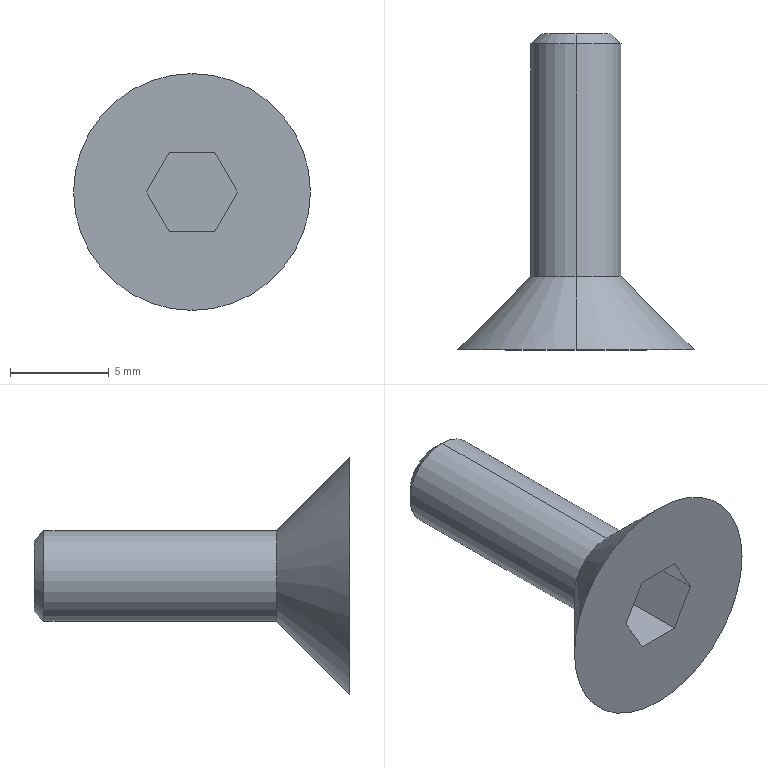Part | CATIA | 1 solid | 15 faces | box 12 x 16 x 12 mm | volume 370.466 mm3 | plane 9 | cone 4 | cylinder 2 | commonest cylinder face diameters 4.6 x2
STEP:
#1=CARTESIAN_POINT('',(0.,0.,-6.));
#2=VERTEX_POINT('',#1);
#3=CARTESIAN_POINT('',(0.,3.7,-2.3));
#4=VERTEX_POINT('',#3);
#5=CARTESIAN_POINT('',(0.,-353549.641,-353555.641));
#6=DIRECTION('',(0.,-0.7071,-0.7071));
#7=VECTOR('',#6,1.);
#8=LINE('',#5,#7);
#9=EDGE_CURVE('',#2,#4,#8,.F.);
#10=ORIENTED_EDGE('',*,*,#9,.F.);
#11=CARTESIAN_POINT('',(0.,0.,6.));
#12=VERTEX_POINT('',#11);
#13=CARTESIAN_POINT('',(0.,0.,0.));
#14=DIRECTION('',(0.,-1.,0.));
#15=AXIS2_PLACEMENT_3D('',#13,#14,$);
#16=CIRCLE('',#15,6.);
#17=EDGE_CURVE('',#2,#12,#16,.F.);
#18=ORIENTED_EDGE('',*,*,#17,.T.);
#19=CARTESIAN_POINT('',(0.,3.7,2.3));
#20=VERTEX_POINT('',#19);
#21=CARTESIAN_POINT('',(0.,-353549.641,353555.641));
#22=DIRECTION('',(0.,-0.7071,0.7071));
#23=VECTOR('',#22,1.);
#24=LINE('',#21,#23);
#25=EDGE_CURVE('',#20,#12,#24,.T.);
#26=ORIENTED_EDGE('',*,*,#25,.F.);
#27=CARTESIAN_POINT('',(0.,3.7,0.));
#28=DIRECTION('',(0.,-1.,0.));
#29=AXIS2_PLACEMENT_3D('',#27,#28,$);
#30=CIRCLE('',#29,2.3);
#31=EDGE_CURVE('',#4,#20,#30,.F.);
#32=ORIENTED_EDGE('',*,*,#31,.F.);
#33=EDGE_LOOP('',(#10,#18,#26,#32));
#34=FACE_OUTER_BOUND('',#33,.T.);
#35=CARTESIAN_POINT('',(0.,1.5,0.));
#36=DIRECTION('',(0.,-1.,0.));
#37=DIRECTION('',(0.,0.,1.));
#38=AXIS2_PLACEMENT_3D('',#35,#36,#37);
#39=CONICAL_SURFACE('',#38,4.5,0.7854);
#40=ADVANCED_FACE('',(#34),#39,.T.);
#41=ORIENTED_EDGE('',*,*,#9,.T.);
#42=CARTESIAN_POINT('',(0.,3.7,0.));
#43=DIRECTION('',(0.,-1.,0.));
#44=AXIS2_PLACEMENT_3D('',#42,#43,$);
#45=CIRCLE('',#44,2.3);
#46=EDGE_CURVE('',#4,#20,#45,.T.);
#47=ORIENTED_EDGE('',*,*,#46,.T.);
#48=ORIENTED_EDGE('',*,*,#25,.T.);
#49=CARTESIAN_POINT('',(0.,0.,0.));
#50=DIRECTION('',(0.,-1.,0.));
#51=AXIS2_PLACEMENT_3D('',#49,#50,$);
#52=CIRCLE('',#51,6.);
#53=EDGE_CURVE('',#12,#2,#52,.F.);
#54=ORIENTED_EDGE('',*,*,#53,.T.);
#55=EDGE_LOOP('',(#41,#47,#48,#54));
#56=FACE_OUTER_BOUND('',#55,.T.);
#57=CARTESIAN_POINT('',(0.,1.5,0.));
#58=DIRECTION('',(0.,-1.,0.));
#59=DIRECTION('',(0.,0.,-1.));
#60=AXIS2_PLACEMENT_3D('',#57,#58,#59);
#61=CONICAL_SURFACE('',#60,4.5,0.7854);
#62=ADVANCED_FACE('',(#56),#61,.T.);
#63=ORIENTED_EDGE('',*,*,#17,.F.);
#64=ORIENTED_EDGE('',*,*,#53,.F.);
#65=EDGE_LOOP('',(#63,#64));
#66=FACE_OUTER_BOUND('',#65,.T.);
#67=CARTESIAN_POINT('',(-2.309,0.,0.));
#68=VERTEX_POINT('',#67);
#69=CARTESIAN_POINT('',(-1.155,0.,2.));
#70=VERTEX_POINT('',#69);
#71=CARTESIAN_POINT('',(-1.732,0.,1.));
#72=DIRECTION('',(0.5,0.,0.866));
#73=VECTOR('',#72,1.);
#74=LINE('',#71,#73);
#75=EDGE_CURVE('',#68,#70,#74,.T.);
#76=ORIENTED_EDGE('',*,*,#75,.T.);
#77=CARTESIAN_POINT('',(1.155,0.,2.));
#78=VERTEX_POINT('',#77);
#79=CARTESIAN_POINT('',(0.,0.,2.));
#80=DIRECTION('',(1.,0.,0.));
#81=VECTOR('',#80,1.);
#82=LINE('',#79,#81);
#83=EDGE_CURVE('',#70,#78,#82,.T.);
#84=ORIENTED_EDGE('',*,*,#83,.T.);
#85=CARTESIAN_POINT('',(2.309,0.,0.));
#86=VERTEX_POINT('',#85);
#87=CARTESIAN_POINT('',(1.732,0.,1.));
#88=DIRECTION('',(0.5,0.,-0.866));
#89=VECTOR('',#88,1.);
#90=LINE('',#87,#89);
#91=EDGE_CURVE('',#78,#86,#90,.T.);
#92=ORIENTED_EDGE('',*,*,#91,.T.);
#93=CARTESIAN_POINT('',(1.155,0.,-2.));
#94=VERTEX_POINT('',#93);
#95=CARTESIAN_POINT('',(1.732,0.,-1.));
#96=DIRECTION('',(-0.5,0.,-0.866));
#97=VECTOR('',#96,1.);
#98=LINE('',#95,#97);
#99=EDGE_CURVE('',#86,#94,#98,.T.);
#100=ORIENTED_EDGE('',*,*,#99,.T.);
#101=CARTESIAN_POINT('',(-1.155,0.,-2.));
#102=VERTEX_POINT('',#101);
#103=CARTESIAN_POINT('',(0.,0.,-2.));
#104=DIRECTION('',(-1.,0.,0.));
#105=VECTOR('',#104,1.);
#106=LINE('',#103,#105);
#107=EDGE_CURVE('',#94,#102,#106,.T.);
#108=ORIENTED_EDGE('',*,*,#107,.T.);
#109=CARTESIAN_POINT('',(-1.732,0.,-1.));
#110=DIRECTION('',(-0.5,0.,0.866));
#111=VECTOR('',#110,1.);
#112=LINE('',#109,#111);
#113=EDGE_CURVE('',#102,#68,#112,.T.);
#114=ORIENTED_EDGE('',*,*,#113,.T.);
#115=EDGE_LOOP('',(#76,#84,#92,#100,#108,#114));
#116=FACE_BOUND('',#115,.T.);
#117=CARTESIAN_POINT('',(0.,0.,-3.));
#118=DIRECTION('',(0.,-1.,0.));
#119=DIRECTION('',(0.,0.,1.));
#120=AXIS2_PLACEMENT_3D('',#117,#118,#119);
#121=PLANE('',#120);
#122=ADVANCED_FACE('',(#66,#116),#121,.T.);
#123=CARTESIAN_POINT('',(-1.155,3.3,2.));
#124=VERTEX_POINT('',#123);
#125=CARTESIAN_POINT('',(-2.309,3.3,0.));
#126=VERTEX_POINT('',#125);
#127=CARTESIAN_POINT('',(-1.732,3.3,1.));
#128=DIRECTION('',(-0.5,0.,-0.866));
#129=VECTOR('',#128,1.);
#130=LINE('',#127,#129);
#131=EDGE_CURVE('',#124,#126,#130,.T.);
#132=ORIENTED_EDGE('',*,*,#131,.F.);
#133=CARTESIAN_POINT('',(-1.155,1.65,2.));
#134=DIRECTION('',(0.,1.,0.));
#135=VECTOR('',#134,1.);
#136=LINE('',#133,#135);
#137=EDGE_CURVE('',#70,#124,#136,.T.);
#138=ORIENTED_EDGE('',*,*,#137,.F.);
#139=ORIENTED_EDGE('',*,*,#75,.F.);
#140=CARTESIAN_POINT('',(-2.309,1.65,0.));
#141=DIRECTION('',(0.,1.,0.));
#142=VECTOR('',#141,1.);
#143=LINE('',#140,#142);
#144=EDGE_CURVE('',#68,#126,#143,.T.);
#145=ORIENTED_EDGE('',*,*,#144,.T.);
#146=EDGE_LOOP('',(#132,#138,#139,#145));
#147=FACE_OUTER_BOUND('',#146,.T.);
#148=CARTESIAN_POINT('',(-1.155,0.,2.));
#149=DIRECTION('',(-0.866,0.,0.5));
#150=DIRECTION('',(0.5,0.,0.866));
#151=AXIS2_PLACEMENT_3D('',#148,#149,#150);
#152=PLANE('',#151);
#153=ADVANCED_FACE('',(#147),#152,.F.);
#154=ORIENTED_EDGE('',*,*,#131,.T.);
#155=CARTESIAN_POINT('',(-1.155,3.3,-2.));
#156=VERTEX_POINT('',#155);
#157=CARTESIAN_POINT('',(-1.732,3.3,-1.));
#158=DIRECTION('',(0.5,0.,-0.866));
#159=VECTOR('',#158,1.);
#160=LINE('',#157,#159);
#161=EDGE_CURVE('',#126,#156,#160,.T.);
#162=ORIENTED_EDGE('',*,*,#161,.T.);
#163=CARTESIAN_POINT('',(1.155,3.3,-2.));
#164=VERTEX_POINT('',#163);
#165=CARTESIAN_POINT('',(0.,3.3,-2.));
#166=DIRECTION('',(1.,0.,0.));
#167=VECTOR('',#166,1.);
#168=LINE('',#165,#167);
#169=EDGE_CURVE('',#156,#164,#168,.T.);
#170=ORIENTED_EDGE('',*,*,#169,.T.);
#171=CARTESIAN_POINT('',(2.309,3.3,0.));
#172=VERTEX_POINT('',#171);
#173=CARTESIAN_POINT('',(1.732,3.3,-1.));
#174=DIRECTION('',(0.5,0.,0.866));
#175=VECTOR('',#174,1.);
#176=LINE('',#173,#175);
#177=EDGE_CURVE('',#164,#172,#176,.T.);
#178=ORIENTED_EDGE('',*,*,#177,.T.);
#179=CARTESIAN_POINT('',(1.155,3.3,2.));
#180=VERTEX_POINT('',#179);
#181=CARTESIAN_POINT('',(1.732,3.3,1.));
#182=DIRECTION('',(-0.5,0.,0.866));
#183=VECTOR('',#182,1.);
#184=LINE('',#181,#183);
#185=EDGE_CURVE('',#172,#180,#184,.T.);
#186=ORIENTED_EDGE('',*,*,#185,.T.);
#187=CARTESIAN_POINT('',(0.,3.3,2.));
#188=DIRECTION('',(-1.,0.,0.));
#189=VECTOR('',#188,1.);
#190=LINE('',#187,#189);
#191=EDGE_CURVE('',#180,#124,#190,.T.);
#192=ORIENTED_EDGE('',*,*,#191,.T.);
#193=EDGE_LOOP('',(#154,#162,#170,#178,#186,#192));
#194=FACE_OUTER_BOUND('',#193,.T.);
#195=CARTESIAN_POINT('',(0.,3.3,0.));
#196=DIRECTION('',(0.,-1.,0.));
#197=DIRECTION('',(0.,0.,-1.));
#198=AXIS2_PLACEMENT_3D('',#195,#196,#197);
#199=PLANE('',#198);
#200=ADVANCED_FACE('',(#194),#199,.T.);
#201=ORIENTED_EDGE('',*,*,#161,.F.);
#202=ORIENTED_EDGE('',*,*,#144,.F.);
#203=ORIENTED_EDGE('',*,*,#113,.F.);
#204=CARTESIAN_POINT('',(-1.155,1.65,-2.));
#205=DIRECTION('',(0.,1.,0.));
#206=VECTOR('',#205,1.);
#207=LINE('',#204,#206);
#208=EDGE_CURVE('',#102,#156,#207,.T.);
#209=ORIENTED_EDGE('',*,*,#208,.T.);
#210=EDGE_LOOP('',(#201,#202,#203,#209));
#211=FACE_OUTER_BOUND('',#210,.T.);
#212=CARTESIAN_POINT('',(-2.309,0.,0.));
#213=DIRECTION('',(-0.866,0.,-0.5));
#214=DIRECTION('',(-0.5,0.,0.866));
#215=AXIS2_PLACEMENT_3D('',#212,#213,#214);
#216=PLANE('',#215);
#217=ADVANCED_FACE('',(#211),#216,.F.);
#218=ORIENTED_EDGE('',*,*,#169,.F.);
#219=ORIENTED_EDGE('',*,*,#208,.F.);
#220=ORIENTED_EDGE('',*,*,#107,.F.);
#221=CARTESIAN_POINT('',(1.155,1.65,-2.));
#222=DIRECTION('',(0.,1.,0.));
#223=VECTOR('',#222,1.);
#224=LINE('',#221,#223);
#225=EDGE_CURVE('',#94,#164,#224,.T.);
#226=ORIENTED_EDGE('',*,*,#225,.T.);
#227=EDGE_LOOP('',(#218,#219,#220,#226));
#228=FACE_OUTER_BOUND('',#227,.T.);
#229=CARTESIAN_POINT('',(-1.155,0.,-2.));
#230=DIRECTION('',(0.,0.,-1.));
#231=DIRECTION('',(-1.,0.,0.));
#232=AXIS2_PLACEMENT_3D('',#229,#230,#231);
#233=PLANE('',#232);
#234=ADVANCED_FACE('',(#228),#233,.F.);
#235=ORIENTED_EDGE('',*,*,#177,.F.);
#236=ORIENTED_EDGE('',*,*,#225,.F.);
#237=ORIENTED_EDGE('',*,*,#99,.F.);
#238=CARTESIAN_POINT('',(2.309,1.65,0.));
#239=DIRECTION('',(0.,1.,0.));
#240=VECTOR('',#239,1.);
#241=LINE('',#238,#240);
#242=EDGE_CURVE('',#86,#172,#241,.T.);
#243=ORIENTED_EDGE('',*,*,#242,.T.);
#244=EDGE_LOOP('',(#235,#236,#237,#243));
#245=FACE_OUTER_BOUND('',#244,.T.);
#246=CARTESIAN_POINT('',(1.155,0.,-2.));
#247=DIRECTION('',(0.866,0.,-0.5));
#248=DIRECTION('',(-0.5,0.,-0.866));
#249=AXIS2_PLACEMENT_3D('',#246,#247,#248);
#250=PLANE('',#249);
#251=ADVANCED_FACE('',(#245),#250,.F.);
#252=ORIENTED_EDGE('',*,*,#185,.F.);
#253=ORIENTED_EDGE('',*,*,#242,.F.);
#254=ORIENTED_EDGE('',*,*,#91,.F.);
#255=CARTESIAN_POINT('',(1.155,1.65,2.));
#256=DIRECTION('',(0.,1.,0.));
#257=VECTOR('',#256,1.);
#258=LINE('',#255,#257);
#259=EDGE_CURVE('',#78,#180,#258,.T.);
#260=ORIENTED_EDGE('',*,*,#259,.T.);
#261=EDGE_LOOP('',(#252,#253,#254,#260));
#262=FACE_OUTER_BOUND('',#261,.T.);
#263=CARTESIAN_POINT('',(2.309,0.,0.));
#264=DIRECTION('',(0.866,0.,0.5));
#265=DIRECTION('',(0.5,0.,-0.866));
#266=AXIS2_PLACEMENT_3D('',#263,#264,#265);
#267=PLANE('',#266);
#268=ADVANCED_FACE('',(#262),#267,.F.);
#269=ORIENTED_EDGE('',*,*,#191,.F.);
#270=ORIENTED_EDGE('',*,*,#259,.F.);
#271=ORIENTED_EDGE('',*,*,#83,.F.);
#272=ORIENTED_EDGE('',*,*,#137,.T.);
#273=EDGE_LOOP('',(#269,#270,#271,#272));
#274=FACE_OUTER_BOUND('',#273,.T.);
#275=CARTESIAN_POINT('',(1.155,0.,2.));
#276=DIRECTION('',(0.,0.,1.));
#277=DIRECTION('',(1.,0.,0.));
#278=AXIS2_PLACEMENT_3D('',#275,#276,#277);
#279=PLANE('',#278);
#280=ADVANCED_FACE('',(#274),#279,.F.);
#281=CARTESIAN_POINT('',(0.,15.5,-2.3));
#282=VERTEX_POINT('',#281);
#283=CARTESIAN_POINT('',(0.,9.9,-2.3));
#284=DIRECTION('',(0.,-1.,0.));
#285=VECTOR('',#284,1.);
#286=LINE('',#283,#285);
#287=EDGE_CURVE('',#4,#282,#286,.F.);
#288=ORIENTED_EDGE('',*,*,#287,.F.);
#289=ORIENTED_EDGE('',*,*,#31,.T.);
#290=CARTESIAN_POINT('',(0.,15.5,2.3));
#291=VERTEX_POINT('',#290);
#292=CARTESIAN_POINT('',(0.,9.9,2.3));
#293=DIRECTION('',(0.,-1.,0.));
#294=VECTOR('',#293,1.);
#295=LINE('',#292,#294);
#296=EDGE_CURVE('',#291,#20,#295,.T.);
#297=ORIENTED_EDGE('',*,*,#296,.F.);
#298=CARTESIAN_POINT('',(0.,15.5,0.));
#299=DIRECTION('',(0.,-1.,0.));
#300=AXIS2_PLACEMENT_3D('',#298,#299,$);
#301=CIRCLE('',#300,2.3);
#302=EDGE_CURVE('',#282,#291,#301,.F.);
#303=ORIENTED_EDGE('',*,*,#302,.F.);
#304=EDGE_LOOP('',(#288,#289,#297,#303));
#305=FACE_OUTER_BOUND('',#304,.T.);
#306=CARTESIAN_POINT('',(0.,9.2,0.));
#307=DIRECTION('',(0.,-1.,0.));
#308=DIRECTION('',(1.,0.,0.));
#309=AXIS2_PLACEMENT_3D('',#306,#307,#308);
#310=CYLINDRICAL_SURFACE('',#309,2.3);
#311=ADVANCED_FACE('',(#305),#310,.T.);
#312=CARTESIAN_POINT('',(-0.000000335,16.,-1.8));
#313=VERTEX_POINT('',#312);
#314=CARTESIAN_POINT('',(0.000000268,16.,1.8));
#315=VERTEX_POINT('',#314);
#316=CARTESIAN_POINT('',(0.,16.,0.));
#317=DIRECTION('',(0.,1.,0.));
#318=AXIS2_PLACEMENT_3D('',#316,#317,$);
#319=CIRCLE('',#318,1.8);
#320=EDGE_CURVE('',#313,#315,#319,.T.);
#321=ORIENTED_EDGE('',*,*,#320,.T.);
#322=CARTESIAN_POINT('',(0.,16.,0.));
#323=DIRECTION('',(0.,1.,0.));
#324=AXIS2_PLACEMENT_3D('',#322,#323,$);
#325=CIRCLE('',#324,1.8);
#326=EDGE_CURVE('',#315,#313,#325,.T.);
#327=ORIENTED_EDGE('',*,*,#326,.T.);
#328=EDGE_LOOP('',(#321,#327));
#329=FACE_OUTER_BOUND('',#328,.T.);
#330=CARTESIAN_POINT('',(0.,16.,-1.2));
#331=DIRECTION('',(0.,1.,0.));
#332=DIRECTION('',(0.,0.,-1.));
#333=AXIS2_PLACEMENT_3D('',#330,#331,#332);
#334=PLANE('',#333);
#335=ADVANCED_FACE('',(#329),#334,.T.);
#336=ORIENTED_EDGE('',*,*,#296,.T.);
#337=ORIENTED_EDGE('',*,*,#46,.F.);
#338=ORIENTED_EDGE('',*,*,#287,.T.);
#339=CARTESIAN_POINT('',(0.,15.5,0.));
#340=DIRECTION('',(0.,-1.,0.));
#341=AXIS2_PLACEMENT_3D('',#339,#340,$);
#342=CIRCLE('',#341,2.3);
#343=EDGE_CURVE('',#291,#282,#342,.F.);
#344=ORIENTED_EDGE('',*,*,#343,.F.);
#345=EDGE_LOOP('',(#336,#337,#338,#344));
#346=FACE_OUTER_BOUND('',#345,.T.);
#347=CARTESIAN_POINT('',(0.,9.2,0.));
#348=DIRECTION('',(0.,-1.,0.));
#349=DIRECTION('',(-1.,0.,0.));
#350=AXIS2_PLACEMENT_3D('',#347,#348,#349);
#351=CYLINDRICAL_SURFACE('',#350,2.3);
#352=ADVANCED_FACE('',(#346),#351,.T.);
#353=CARTESIAN_POINT('',(0.,15.75,-2.05));
#354=DIRECTION('',(0.,-0.7071,-0.7071));
#355=VECTOR('',#354,1.);
#356=LINE('',#353,#355);
#357=EDGE_CURVE('',#313,#282,#356,.T.);
#358=ORIENTED_EDGE('',*,*,#357,.T.);
#359=ORIENTED_EDGE('',*,*,#302,.T.);
#360=CARTESIAN_POINT('',(0.,15.75,2.05));
#361=DIRECTION('',(0.,-0.7071,0.7071));
#362=VECTOR('',#361,1.);
#363=LINE('',#360,#362);
#364=EDGE_CURVE('',#315,#291,#363,.T.);
#365=ORIENTED_EDGE('',*,*,#364,.F.);
#366=ORIENTED_EDGE('',*,*,#320,.F.);
#367=EDGE_LOOP('',(#358,#359,#365,#366));
#368=FACE_OUTER_BOUND('',#367,.T.);
#369=CARTESIAN_POINT('',(0.,17.8,0.));
#370=DIRECTION('',(0.,-1.,0.));
#371=DIRECTION('',(0.1243,0.,-0.9923));
#372=AXIS2_PLACEMENT_3D('',#369,#370,#371);
#373=CONICAL_SURFACE('',#372,0.,0.7854);
#374=ADVANCED_FACE('',(#368),#373,.T.);
#375=ORIENTED_EDGE('',*,*,#364,.T.);
#376=ORIENTED_EDGE('',*,*,#343,.T.);
#377=ORIENTED_EDGE('',*,*,#357,.F.);
#378=ORIENTED_EDGE('',*,*,#326,.F.);
#379=EDGE_LOOP('',(#375,#376,#377,#378));
#380=FACE_OUTER_BOUND('',#379,.T.);
#381=CARTESIAN_POINT('',(0.,17.8,0.));
#382=DIRECTION('',(0.,-1.,0.));
#383=DIRECTION('',(-0.5878,0.,0.809));
#384=AXIS2_PLACEMENT_3D('',#381,#382,#383);
#385=CONICAL_SURFACE('',#384,0.,0.7854);
#386=ADVANCED_FACE('',(#380),#385,.T.);
#387=CLOSED_SHELL('',(#40,#62,#122,#153,#200,#217,#234,#251,#268,#280,#311,#335,#352,#374,#386));
#388=MANIFOLD_SOLID_BREP('',#387);
#389=(LENGTH_UNIT()NAMED_UNIT(*)SI_UNIT(.MILLI.,.METRE.));
#390=UNCERTAINTY_MEASURE_WITH_UNIT(LENGTH_MEASURE(0.005),#389,'','');
#391=(NAMED_UNIT(*)PLANE_ANGLE_UNIT()SI_UNIT($,.RADIAN.));
#392=(NAMED_UNIT(*)SI_UNIT($,.STERADIAN.)SOLID_ANGLE_UNIT());
#393=(GEOMETRIC_REPRESENTATION_CONTEXT(3)GLOBAL_UNCERTAINTY_ASSIGNED_CONTEXT((#390))GLOBAL_UNIT_ASSIGNED_CONTEXT((#389,#391,#392))REPRESENTATION_CONTEXT('',''));
#394=ADVANCED_BREP_SHAPE_REPRESENTATION('',(#388),#393);